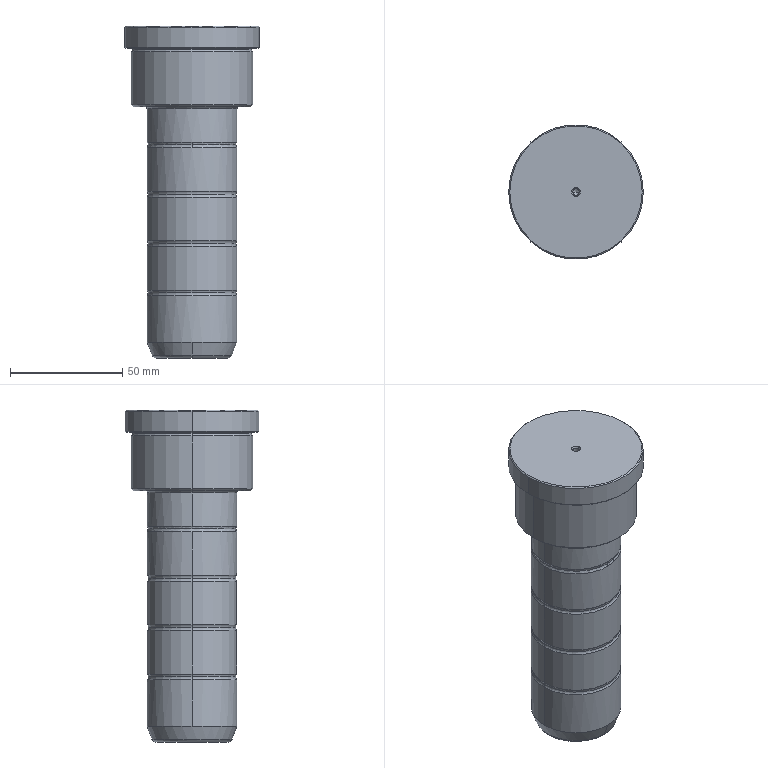Part | STEP file | Upper pillar C- PN_0004 - cut | 1 solid | 64 faces | box 60 x 60 x 148 mm | volume 226817 mm3 | torus 24 | cone 18 | cylinder 18 | plane 4 | commonest cylinder face diameters 40 x10 3 x4 54 x2 60 x2